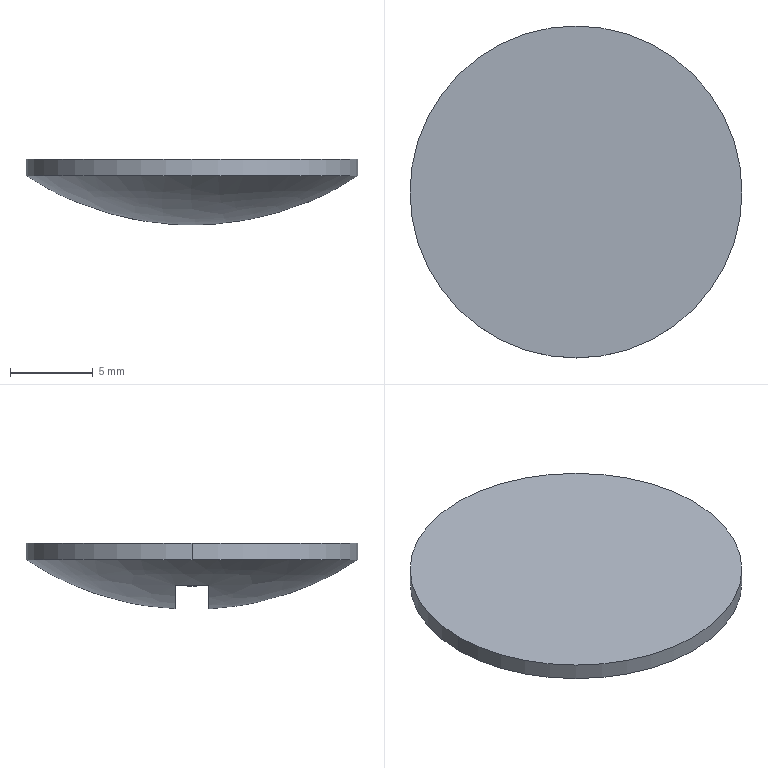Part | SolidWorks | features BaseBody 1 | 1 solid | 9 faces | box 20 x 20 x 3.972 mm | volume 728.686 mm3 | plane 6 | cylinder 2 | spline 1 | commonest cylinder face diameters 20 x2
STEP:
#1=CARTESIAN_POINT('',(363.,-93.,-56.087));
#2=VERTEX_POINT('',#1);
#3=CARTESIAN_POINT('',(343.,-93.,-56.087));
#4=VERTEX_POINT('',#3);
#5=CARTESIAN_POINT('',(353.,-93.,-56.087));
#6=DIRECTION('',(0.,0.,1.));
#7=DIRECTION('',(-1.,0.,0.));
#8=AXIS2_PLACEMENT_3D('',#5,#6,#7);
#9=CIRCLE('',#8,10.);
#10=EDGE_CURVE('',#2,#4,#9,.T.);
#11=ORIENTED_EDGE('',*,*,#10,.F.);
#12=CARTESIAN_POINT('',(363.,-93.,-57.087));
#13=VERTEX_POINT('',#12);
#14=CARTESIAN_POINT('',(363.,-93.,-56.587));
#15=DIRECTION('',(0.,0.,-1.));
#16=VECTOR('',#15,1000.);
#17=LINE('',#14,#16);
#18=EDGE_CURVE('',#2,#13,#17,.T.);
#19=ORIENTED_EDGE('',*,*,#18,.T.);
#20=CARTESIAN_POINT('',(343.,-93.,-57.087));
#21=VERTEX_POINT('',#20);
#22=CARTESIAN_POINT('',(353.,-93.,-57.087));
#23=DIRECTION('',(0.,0.,1.));
#24=DIRECTION('',(-1.,0.,0.));
#25=AXIS2_PLACEMENT_3D('',#22,#23,#24);
#26=CIRCLE('',#25,10.);
#27=EDGE_CURVE('',#13,#21,#26,.T.);
#28=ORIENTED_EDGE('',*,*,#27,.T.);
#29=CARTESIAN_POINT('',(343.,-93.,-56.587));
#30=DIRECTION('',(0.,0.,-1.));
#31=VECTOR('',#30,1000.);
#32=LINE('',#29,#31);
#33=EDGE_CURVE('',#4,#21,#32,.T.);
#34=ORIENTED_EDGE('',*,*,#33,.F.);
#35=EDGE_LOOP('',(#11,#19,#28,#34));
#36=FACE_OUTER_BOUND('',#35,.T.);
#37=CARTESIAN_POINT('',(353.,-93.,-56.587));
#38=DIRECTION('',(0.,0.,-1.));
#39=DIRECTION('',(-1.,0.,0.));
#40=AXIS2_PLACEMENT_3D('',#37,#38,#39);
#41=CYLINDRICAL_SURFACE('',#40,10.);
#42=ADVANCED_FACE('',(#36),#41,.T.);
#43=CARTESIAN_POINT('',(353.,-93.,-56.087));
#44=DIRECTION('',(0.,0.,1.));
#45=DIRECTION('',(-1.,0.,0.));
#46=AXIS2_PLACEMENT_3D('',#43,#44,#45);
#47=CIRCLE('',#46,10.);
#48=EDGE_CURVE('',#4,#2,#47,.T.);
#49=ORIENTED_EDGE('',*,*,#48,.T.);
#50=ORIENTED_EDGE('',*,*,#10,.T.);
#51=EDGE_LOOP('',(#49,#50));
#52=FACE_OUTER_BOUND('',#51,.T.);
#53=CARTESIAN_POINT('',(358.,-93.,-56.087));
#54=DIRECTION('',(0.,0.,1.));
#55=DIRECTION('',(1.,0.,0.));
#56=AXIS2_PLACEMENT_3D('',#53,#54,#55);
#57=PLANE('',#56);
#58=ADVANCED_FACE('',(#52),#57,.T.);
#59=ORIENTED_EDGE('',*,*,#18,.F.);
#60=ORIENTED_EDGE('',*,*,#48,.F.);
#61=ORIENTED_EDGE('',*,*,#33,.T.);
#62=CARTESIAN_POINT('',(353.,-93.,-57.087));
#63=DIRECTION('',(0.,0.,1.));
#64=DIRECTION('',(-1.,0.,0.));
#65=AXIS2_PLACEMENT_3D('',#62,#63,#64);
#66=CIRCLE('',#65,10.);
#67=EDGE_CURVE('',#21,#13,#66,.T.);
#68=ORIENTED_EDGE('',*,*,#67,.T.);
#69=EDGE_LOOP('',(#59,#60,#61,#68));
#70=FACE_OUTER_BOUND('',#69,.T.);
#71=CARTESIAN_POINT('',(353.,-93.,-56.587));
#72=DIRECTION('',(0.,0.,-1.));
#73=DIRECTION('',(-1.,0.,0.));
#74=AXIS2_PLACEMENT_3D('',#71,#72,#73);
#75=CYLINDRICAL_SURFACE('',#74,10.);
#76=ADVANCED_FACE('',(#70),#75,.T.);
#77=CARTESIAN_POINT('',(346.,-94.,-58.654));
#78=VERTEX_POINT('',#77);
#79=CARTESIAN_POINT('',(346.,-92.,-58.654));
#80=VERTEX_POINT('',#79);
#81=CARTESIAN_POINT('',(346.,-94.,-58.654));
#82=CARTESIAN_POINT('',(346.,-93.334,-58.694));
#83=CARTESIAN_POINT('',(346.,-92.666,-58.694));
#84=CARTESIAN_POINT('',(346.,-92.,-58.654));
#85=B_SPLINE_CURVE_WITH_KNOTS('',3,(#81,#82,#83,#84),.UNSPECIFIED.,.F.,.F.,(4,4),(-0.001,0.001),.UNSPECIFIED.);
#86=EDGE_CURVE('',#78,#80,#85,.T.);
#87=ORIENTED_EDGE('',*,*,#86,.F.);
#88=CARTESIAN_POINT('',(360.,-94.,-58.654));
#89=VERTEX_POINT('',#88);
#90=CARTESIAN_POINT('',(346.,-94.,-58.654));
#91=CARTESIAN_POINT('',(347.12,-94.,-59.123));
#92=CARTESIAN_POINT('',(349.407,-94.,-59.818));
#93=CARTESIAN_POINT('',(351.786,-94.,-60.059));
#94=CARTESIAN_POINT('',(354.214,-94.,-60.059));
#95=CARTESIAN_POINT('',(356.593,-94.,-59.818));
#96=CARTESIAN_POINT('',(358.88,-94.,-59.123));
#97=CARTESIAN_POINT('',(360.,-94.,-58.654));
#98=B_SPLINE_CURVE_WITH_KNOTS('',3,(#90,#91,#92,#93,#94,#95,#96,#97),.UNSPECIFIED.,.F.,.F.,(4,1,2,1,4),(-0.00714,-0.00357,0.,0.00357,0.00714),.UNSPECIFIED.);
#99=EDGE_CURVE('',#78,#89,#98,.T.);
#100=ORIENTED_EDGE('',*,*,#99,.T.);
#101=CARTESIAN_POINT('',(360.,-92.,-58.654));
#102=VERTEX_POINT('',#101);
#103=CARTESIAN_POINT('',(360.,-92.,-58.654));
#104=CARTESIAN_POINT('',(360.,-92.666,-58.694));
#105=CARTESIAN_POINT('',(360.,-93.334,-58.694));
#106=CARTESIAN_POINT('',(360.,-94.,-58.654));
#107=B_SPLINE_CURVE_WITH_KNOTS('',3,(#103,#104,#105,#106),.UNSPECIFIED.,.F.,.F.,(4,4),(-0.001,0.001),.UNSPECIFIED.);
#108=EDGE_CURVE('',#102,#89,#107,.T.);
#109=ORIENTED_EDGE('',*,*,#108,.F.);
#110=CARTESIAN_POINT('',(360.,-92.,-58.654));
#111=CARTESIAN_POINT('',(358.886,-92.,-59.12));
#112=CARTESIAN_POINT('',(357.744,-92.,-59.469));
#113=CARTESIAN_POINT('',(355.993,-92.,-59.821));
#114=CARTESIAN_POINT('',(355.402,-92.,-59.91));
#115=CARTESIAN_POINT('',(354.208,-92.,-60.029));
#116=CARTESIAN_POINT('',(353.602,-92.,-60.059));
#117=CARTESIAN_POINT('',(351.806,-92.,-60.06));
#118=CARTESIAN_POINT('',(350.621,-92.,-59.942));
#119=CARTESIAN_POINT('',(348.863,-92.,-59.591));
#120=CARTESIAN_POINT('',(348.278,-92.,-59.444));
#121=CARTESIAN_POINT('',(347.124,-92.,-59.092));
#122=CARTESIAN_POINT('',(346.557,-92.,-58.887));
#123=CARTESIAN_POINT('',(346.,-92.,-58.654));
#124=B_SPLINE_CURVE_WITH_KNOTS('',3,(#110,#111,#112,#113,#114,#115,#116,#117,#118,#119,#120,#121,#122,#123),.UNSPECIFIED.,.F.,.F.,(4,2,2,2,2,2,4),(0.,0.003572,0.005358,0.007144,0.01072,0.0125,0.01429),.UNSPECIFIED.);
#125=EDGE_CURVE('',#102,#80,#124,.T.);
#126=ORIENTED_EDGE('',*,*,#125,.T.);
#127=EDGE_LOOP('',(#87,#100,#109,#126));
#128=FACE_BOUND('',#127,.T.);
#129=ORIENTED_EDGE('',*,*,#67,.F.);
#130=ORIENTED_EDGE('',*,*,#27,.F.);
#131=EDGE_LOOP('',(#129,#130));
#132=FACE_OUTER_BOUND('',#131,.T.);
#133=CARTESIAN_POINT('',(344.29,-82.228,-53.673));
#134=CARTESIAN_POINT('',(342.35,-88.864,-58.317));
#135=CARTESIAN_POINT('',(342.355,-97.192,-58.306));
#136=CARTESIAN_POINT('',(344.302,-103.813,-53.644));
#137=CARTESIAN_POINT('',(350.748,-81.337,-57.643));
#138=CARTESIAN_POINT('',(348.648,-88.522,-62.671));
#139=CARTESIAN_POINT('',(348.653,-97.539,-62.659));
#140=CARTESIAN_POINT('',(350.761,-104.707,-57.612));
#141=CARTESIAN_POINT('',(358.149,-83.126,-58.177));
#142=CARTESIAN_POINT('',(356.371,-89.209,-62.434));
#143=CARTESIAN_POINT('',(356.376,-96.842,-62.424));
#144=CARTESIAN_POINT('',(358.16,-102.911,-58.151));
#145=CARTESIAN_POINT('',(363.968,-86.985,-55.094));
#146=CARTESIAN_POINT('',(362.885,-90.69,-57.687));
#147=CARTESIAN_POINT('',(362.888,-95.341,-57.681));
#148=CARTESIAN_POINT('',(363.975,-99.038,-55.078));
#149=(BOUNDED_SURFACE()B_SPLINE_SURFACE(3,3,((#133,#134,#135,#136),(#137,#138,#139,#140),(#141,#142,#143,#144),(#145,#146,#147,#148)),.UNSPECIFIED.,.F.,.F.,.T.)B_SPLINE_SURFACE_WITH_KNOTS((4,4),(4,4),(0.,1.),(0.,1.),.UNSPECIFIED.)GEOMETRIC_REPRESENTATION_ITEM()RATIONAL_B_SPLINE_SURFACE(((1.,0.8639,0.8639,1.),(0.8863,0.7657,0.7657,0.8863),(0.8863,0.7657,0.7657,0.8863),(1.,0.8639,0.8639,1.)))REPRESENTATION_ITEM('')SURFACE());
#150=ADVANCED_FACE('',(#128,#132),#149,.T.);
#151=CARTESIAN_POINT('',(360.,-94.,-57.087));
#152=VERTEX_POINT('',#151);
#153=CARTESIAN_POINT('',(360.,-94.,-59.087));
#154=DIRECTION('',(0.,0.,1.));
#155=VECTOR('',#154,1000.);
#156=LINE('',#153,#155);
#157=EDGE_CURVE('',#89,#152,#156,.T.);
#158=ORIENTED_EDGE('',*,*,#157,.F.);
#159=ORIENTED_EDGE('',*,*,#99,.F.);
#160=CARTESIAN_POINT('',(346.,-94.,-57.087));
#161=VERTEX_POINT('',#160);
#162=CARTESIAN_POINT('',(346.,-94.,-59.087));
#163=DIRECTION('',(0.,0.,-1.));
#164=VECTOR('',#163,1000.);
#165=LINE('',#162,#164);
#166=EDGE_CURVE('',#161,#78,#165,.T.);
#167=ORIENTED_EDGE('',*,*,#166,.F.);
#168=CARTESIAN_POINT('',(353.,-94.,-57.087));
#169=DIRECTION('',(1.,0.,0.));
#170=VECTOR('',#169,1000.);
#171=LINE('',#168,#170);
#172=EDGE_CURVE('',#161,#152,#171,.T.);
#173=ORIENTED_EDGE('',*,*,#172,.T.);
#174=EDGE_LOOP('',(#158,#159,#167,#173));
#175=FACE_OUTER_BOUND('',#174,.T.);
#176=CARTESIAN_POINT('',(353.,-94.,-59.087));
#177=DIRECTION('',(0.,1.,0.));
#178=DIRECTION('',(0.,0.,1.));
#179=AXIS2_PLACEMENT_3D('',#176,#177,#178);
#180=PLANE('',#179);
#181=ADVANCED_FACE('',(#175),#180,.T.);
#182=CARTESIAN_POINT('',(346.,-92.,-57.087));
#183=VERTEX_POINT('',#182);
#184=CARTESIAN_POINT('',(346.,-92.,-59.087));
#185=DIRECTION('',(0.,0.,1.));
#186=VECTOR('',#185,1000.);
#187=LINE('',#184,#186);
#188=EDGE_CURVE('',#80,#183,#187,.T.);
#189=ORIENTED_EDGE('',*,*,#188,.F.);
#190=ORIENTED_EDGE('',*,*,#125,.F.);
#191=CARTESIAN_POINT('',(360.,-92.,-57.087));
#192=VERTEX_POINT('',#191);
#193=CARTESIAN_POINT('',(360.,-92.,-59.087));
#194=DIRECTION('',(0.,0.,-1.));
#195=VECTOR('',#194,1000.);
#196=LINE('',#193,#195);
#197=EDGE_CURVE('',#192,#102,#196,.T.);
#198=ORIENTED_EDGE('',*,*,#197,.F.);
#199=CARTESIAN_POINT('',(353.,-92.,-57.087));
#200=DIRECTION('',(-1.,0.,0.));
#201=VECTOR('',#200,1000.);
#202=LINE('',#199,#201);
#203=EDGE_CURVE('',#192,#183,#202,.T.);
#204=ORIENTED_EDGE('',*,*,#203,.T.);
#205=EDGE_LOOP('',(#189,#190,#198,#204));
#206=FACE_OUTER_BOUND('',#205,.T.);
#207=CARTESIAN_POINT('',(353.,-92.,-59.087));
#208=DIRECTION('',(0.,-1.,0.));
#209=DIRECTION('',(0.,0.,-1.));
#210=AXIS2_PLACEMENT_3D('',#207,#208,#209);
#211=PLANE('',#210);
#212=ADVANCED_FACE('',(#206),#211,.T.);
#213=ORIENTED_EDGE('',*,*,#203,.F.);
#214=CARTESIAN_POINT('',(360.,-93.,-57.087));
#215=DIRECTION('',(0.,-1.,0.));
#216=VECTOR('',#215,1000.);
#217=LINE('',#214,#216);
#218=EDGE_CURVE('',#192,#152,#217,.T.);
#219=ORIENTED_EDGE('',*,*,#218,.T.);
#220=ORIENTED_EDGE('',*,*,#172,.F.);
#221=CARTESIAN_POINT('',(346.,-93.,-57.087));
#222=DIRECTION('',(0.,1.,0.));
#223=VECTOR('',#222,1000.);
#224=LINE('',#221,#223);
#225=EDGE_CURVE('',#161,#183,#224,.T.);
#226=ORIENTED_EDGE('',*,*,#225,.T.);
#227=EDGE_LOOP('',(#213,#219,#220,#226));
#228=FACE_OUTER_BOUND('',#227,.T.);
#229=CARTESIAN_POINT('',(353.,-93.,-57.087));
#230=DIRECTION('',(0.,0.,-1.));
#231=DIRECTION('',(-1.,0.,0.));
#232=AXIS2_PLACEMENT_3D('',#229,#230,#231);
#233=PLANE('',#232);
#234=ADVANCED_FACE('',(#228),#233,.T.);
#235=ORIENTED_EDGE('',*,*,#197,.T.);
#236=ORIENTED_EDGE('',*,*,#108,.T.);
#237=ORIENTED_EDGE('',*,*,#157,.T.);
#238=ORIENTED_EDGE('',*,*,#218,.F.);
#239=EDGE_LOOP('',(#235,#236,#237,#238));
#240=FACE_OUTER_BOUND('',#239,.T.);
#241=CARTESIAN_POINT('',(360.,-93.,-59.087));
#242=DIRECTION('',(-1.,0.,0.));
#243=DIRECTION('',(0.,0.,1.));
#244=AXIS2_PLACEMENT_3D('',#241,#242,#243);
#245=PLANE('',#244);
#246=ADVANCED_FACE('',(#240),#245,.T.);
#247=ORIENTED_EDGE('',*,*,#166,.T.);
#248=ORIENTED_EDGE('',*,*,#86,.T.);
#249=ORIENTED_EDGE('',*,*,#188,.T.);
#250=ORIENTED_EDGE('',*,*,#225,.F.);
#251=EDGE_LOOP('',(#247,#248,#249,#250));
#252=FACE_OUTER_BOUND('',#251,.T.);
#253=CARTESIAN_POINT('',(346.,-93.,-59.087));
#254=DIRECTION('',(1.,0.,0.));
#255=DIRECTION('',(0.,0.,-1.));
#256=AXIS2_PLACEMENT_3D('',#253,#254,#255);
#257=PLANE('',#256);
#258=ADVANCED_FACE('',(#252),#257,.T.);
#259=CLOSED_SHELL('',(#42,#58,#76,#150,#181,#212,#234,#246,#258));
#260=MANIFOLD_SOLID_BREP('',#259);
#261=CARTESIAN_POINT('',(0.,0.,0.));
#262=DIRECTION('',(0.,0.,1.));
#263=DIRECTION('',(1.,0.,0.));
#264=AXIS2_PLACEMENT_3D('',#261,#262,#263);
#265=(LENGTH_UNIT()NAMED_UNIT(*)SI_UNIT(.MILLI.,.METRE.));
#266=UNCERTAINTY_MEASURE_WITH_UNIT(LENGTH_MEASURE(0.00001),#265,'','');
#267=(NAMED_UNIT(*)PLANE_ANGLE_UNIT()SI_UNIT($,.RADIAN.));
#268=(NAMED_UNIT(*)SI_UNIT($,.STERADIAN.)SOLID_ANGLE_UNIT());
#269=(GEOMETRIC_REPRESENTATION_CONTEXT(3)GLOBAL_UNCERTAINTY_ASSIGNED_CONTEXT((#266))GLOBAL_UNIT_ASSIGNED_CONTEXT((#265,#267,#268))REPRESENTATION_CONTEXT('',''));
#270=ADVANCED_BREP_SHAPE_REPRESENTATION('',(#260,#264),#269);